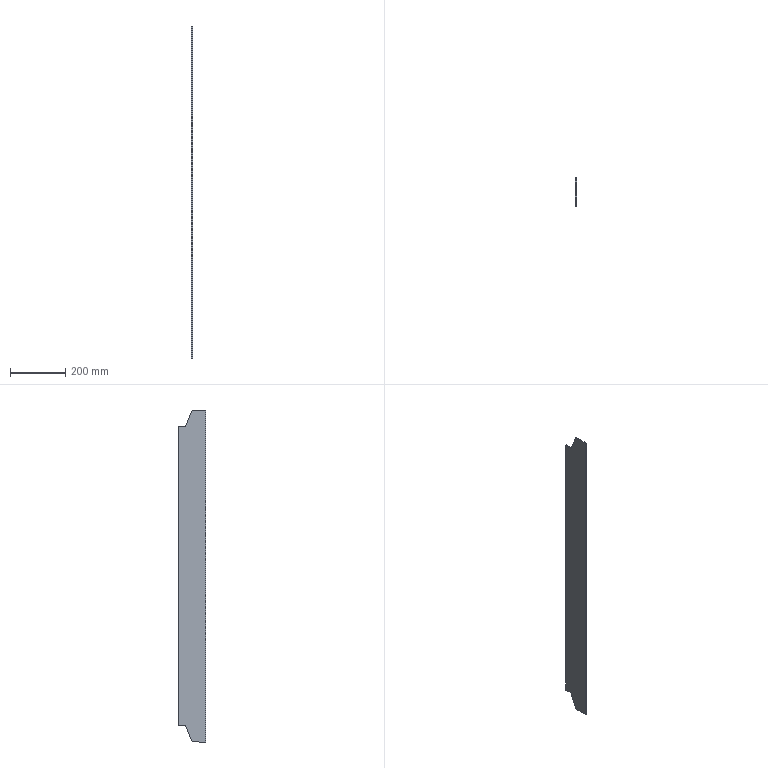Part | SolidWorks | features BaseBody 1 | 1 solid | 10 faces | box 3.795 x 101.02 x 1200 mm | volume 442400 mm3 | plane 9 | cylinder 1 | commonest cylinder face diameters 22.084 x1
STEP:
#1=CARTESIAN_POINT('',(-1.898,-111.897,-1200.));
#2=VERTEX_POINT('',#1);
#3=CARTESIAN_POINT('',(-1.898,-111.897,0.));
#4=VERTEX_POINT('',#3);
#5=CARTESIAN_POINT('',(-1.898,-111.897,0.));
#6=DIRECTION('',(0.,0.,1.));
#7=VECTOR('',#6,1000.);
#8=LINE('',#5,#7);
#9=EDGE_CURVE('',#2,#4,#8,.T.);
#10=ORIENTED_EDGE('',*,*,#9,.T.);
#11=CARTESIAN_POINT('',(-1.898,-61.387,0.));
#12=VERTEX_POINT('',#11);
#13=CARTESIAN_POINT('',(-1.898,-111.897,0.));
#14=DIRECTION('',(0.,1.,0.));
#15=VECTOR('',#14,1000.);
#16=LINE('',#13,#15);
#17=EDGE_CURVE('',#4,#12,#16,.T.);
#18=ORIENTED_EDGE('',*,*,#17,.T.);
#19=CARTESIAN_POINT('',(-1.898,-38.186,-58.335));
#20=VERTEX_POINT('',#19);
#21=CARTESIAN_POINT('',(-1.898,-61.387,0.));
#22=DIRECTION('',(0.,0.3696,-0.9292));
#23=VECTOR('',#22,1000.);
#24=LINE('',#21,#23);
#25=EDGE_CURVE('',#12,#20,#24,.T.);
#26=ORIENTED_EDGE('',*,*,#25,.T.);
#27=CARTESIAN_POINT('',(-1.898,-10.878,-58.335));
#28=VERTEX_POINT('',#27);
#29=CARTESIAN_POINT('',(-1.898,-111.897,-58.335));
#30=DIRECTION('',(0.,1.,0.));
#31=VECTOR('',#30,1000.);
#32=LINE('',#29,#31);
#33=EDGE_CURVE('',#20,#28,#32,.T.);
#34=ORIENTED_EDGE('',*,*,#33,.T.);
#35=CARTESIAN_POINT('',(-1.898,-10.878,-1141.665));
#36=VERTEX_POINT('',#35);
#37=CARTESIAN_POINT('',(-1.898,-10.878,0.));
#38=DIRECTION('',(0.,0.,-1.));
#39=VECTOR('',#38,1000.);
#40=LINE('',#37,#39);
#41=EDGE_CURVE('',#28,#36,#40,.T.);
#42=ORIENTED_EDGE('',*,*,#41,.T.);
#43=CARTESIAN_POINT('',(-1.898,-38.186,-1141.665));
#44=VERTEX_POINT('',#43);
#45=CARTESIAN_POINT('',(-1.898,-111.897,-1141.665));
#46=DIRECTION('',(0.,-1.,0.));
#47=VECTOR('',#46,1000.);
#48=LINE('',#45,#47);
#49=EDGE_CURVE('',#36,#44,#48,.T.);
#50=ORIENTED_EDGE('',*,*,#49,.T.);
#51=CARTESIAN_POINT('',(-1.898,-61.387,-1200.));
#52=VERTEX_POINT('',#51);
#53=CARTESIAN_POINT('',(-1.898,-38.186,-1141.665));
#54=DIRECTION('',(0.,-0.3696,-0.9292));
#55=VECTOR('',#54,1000.);
#56=LINE('',#53,#55);
#57=EDGE_CURVE('',#44,#52,#56,.T.);
#58=ORIENTED_EDGE('',*,*,#57,.T.);
#59=CARTESIAN_POINT('',(-1.898,-111.897,-1200.));
#60=DIRECTION('',(0.,-1.,0.));
#61=VECTOR('',#60,1000.);
#62=LINE('',#59,#61);
#63=EDGE_CURVE('',#52,#2,#62,.T.);
#64=ORIENTED_EDGE('',*,*,#63,.T.);
#65=EDGE_LOOP('',(#10,#18,#26,#34,#42,#50,#58,#64));
#66=FACE_OUTER_BOUND('',#65,.T.);
#67=CARTESIAN_POINT('',(-1.898,-111.897,0.));
#68=DIRECTION('',(-1.,0.,0.));
#69=DIRECTION('',(0.,-1.,0.));
#70=AXIS2_PLACEMENT_3D('',#67,#68,#69);
#71=PLANE('',#70);
#72=ADVANCED_FACE('',(#66),#71,.T.);
#73=CARTESIAN_POINT('',(1.898,-111.897,0.));
#74=VERTEX_POINT('',#73);
#75=CARTESIAN_POINT('',(0.,-111.897,0.));
#76=DIRECTION('',(1.,0.,0.));
#77=VECTOR('',#76,1000.);
#78=LINE('',#75,#77);
#79=EDGE_CURVE('',#4,#74,#78,.T.);
#80=ORIENTED_EDGE('',*,*,#79,.T.);
#81=CARTESIAN_POINT('',(1.898,-61.387,0.));
#82=VERTEX_POINT('',#81);
#83=CARTESIAN_POINT('',(1.898,-61.387,0.));
#84=DIRECTION('',(0.,1.,0.));
#85=VECTOR('',#84,1000.);
#86=LINE('',#83,#85);
#87=EDGE_CURVE('',#74,#82,#86,.T.);
#88=ORIENTED_EDGE('',*,*,#87,.T.);
#89=CARTESIAN_POINT('',(0.,-61.387,0.));
#90=DIRECTION('',(-1.,0.,0.));
#91=VECTOR('',#90,1000.);
#92=LINE('',#89,#91);
#93=EDGE_CURVE('',#82,#12,#92,.T.);
#94=ORIENTED_EDGE('',*,*,#93,.T.);
#95=ORIENTED_EDGE('',*,*,#17,.F.);
#96=EDGE_LOOP('',(#80,#88,#94,#95));
#97=FACE_OUTER_BOUND('',#96,.T.);
#98=CARTESIAN_POINT('',(0.,-61.387,0.));
#99=DIRECTION('',(0.,0.,1.));
#100=DIRECTION('',(1.,0.,0.));
#101=AXIS2_PLACEMENT_3D('',#98,#99,#100);
#102=PLANE('',#101);
#103=ADVANCED_FACE('',(#97),#102,.T.);
#104=CARTESIAN_POINT('',(1.898,-111.897,-1200.));
#105=VERTEX_POINT('',#104);
#106=CARTESIAN_POINT('',(1.898,-111.897,-1200.));
#107=DIRECTION('',(1.,0.,0.));
#108=VECTOR('',#107,1000.);
#109=LINE('',#106,#108);
#110=EDGE_CURVE('',#2,#105,#109,.T.);
#111=ORIENTED_EDGE('',*,*,#110,.T.);
#112=CARTESIAN_POINT('',(1.898,-111.897,0.));
#113=DIRECTION('',(0.,0.,1.));
#114=VECTOR('',#113,1000.);
#115=LINE('',#112,#114);
#116=EDGE_CURVE('',#105,#74,#115,.T.);
#117=ORIENTED_EDGE('',*,*,#116,.T.);
#118=ORIENTED_EDGE('',*,*,#79,.F.);
#119=ORIENTED_EDGE('',*,*,#9,.F.);
#120=EDGE_LOOP('',(#111,#117,#118,#119));
#121=FACE_OUTER_BOUND('',#120,.T.);
#122=CARTESIAN_POINT('',(1.898,-111.897,0.));
#123=DIRECTION('',(0.,-1.,0.));
#124=DIRECTION('',(0.,0.,-1.));
#125=AXIS2_PLACEMENT_3D('',#122,#123,#124);
#126=PLANE('',#125);
#127=ADVANCED_FACE('',(#121),#126,.T.);
#128=CARTESIAN_POINT('',(1.898,-61.387,-1200.));
#129=VERTEX_POINT('',#128);
#130=CARTESIAN_POINT('',(1.898,-61.387,-1200.));
#131=DIRECTION('',(0.,1.,0.));
#132=VECTOR('',#131,1000.);
#133=LINE('',#130,#132);
#134=EDGE_CURVE('',#105,#129,#133,.T.);
#135=ORIENTED_EDGE('',*,*,#134,.F.);
#136=ORIENTED_EDGE('',*,*,#110,.F.);
#137=ORIENTED_EDGE('',*,*,#63,.F.);
#138=CARTESIAN_POINT('',(0.,-61.387,-1200.));
#139=DIRECTION('',(-1.,0.,0.));
#140=VECTOR('',#139,1000.);
#141=LINE('',#138,#140);
#142=EDGE_CURVE('',#129,#52,#141,.T.);
#143=ORIENTED_EDGE('',*,*,#142,.F.);
#144=EDGE_LOOP('',(#135,#136,#137,#143));
#145=FACE_OUTER_BOUND('',#144,.T.);
#146=CARTESIAN_POINT('',(0.,-61.387,-1200.));
#147=DIRECTION('',(0.,0.,1.));
#148=DIRECTION('',(1.,0.,0.));
#149=AXIS2_PLACEMENT_3D('',#146,#147,#148);
#150=PLANE('',#149);
#151=ADVANCED_FACE('',(#145),#150,.F.);
#152=ORIENTED_EDGE('',*,*,#142,.T.);
#153=ORIENTED_EDGE('',*,*,#57,.F.);
#154=CARTESIAN_POINT('',(1.898,-38.186,-1141.665));
#155=VERTEX_POINT('',#154);
#156=CARTESIAN_POINT('',(-1.898,-38.186,-1141.665));
#157=DIRECTION('',(-1.,0.,0.));
#158=VECTOR('',#157,1000.);
#159=LINE('',#156,#158);
#160=EDGE_CURVE('',#155,#44,#159,.T.);
#161=ORIENTED_EDGE('',*,*,#160,.F.);
#162=CARTESIAN_POINT('',(1.898,-38.186,-1141.665));
#163=DIRECTION('',(0.,0.3696,0.9292));
#164=VECTOR('',#163,1000.);
#165=LINE('',#162,#164);
#166=EDGE_CURVE('',#129,#155,#165,.T.);
#167=ORIENTED_EDGE('',*,*,#166,.F.);
#168=EDGE_LOOP('',(#152,#153,#161,#167));
#169=FACE_OUTER_BOUND('',#168,.T.);
#170=CARTESIAN_POINT('',(-1.898,-38.186,-1141.665));
#171=DIRECTION('',(0.,-0.9292,0.3696));
#172=DIRECTION('',(0.,-0.3696,-0.9292));
#173=AXIS2_PLACEMENT_3D('',#170,#171,#172);
#174=PLANE('',#173);
#175=ADVANCED_FACE('',(#169),#174,.F.);
#176=ORIENTED_EDGE('',*,*,#160,.T.);
#177=ORIENTED_EDGE('',*,*,#49,.F.);
#178=CARTESIAN_POINT('',(1.898,-10.878,-1141.665));
#179=VERTEX_POINT('',#178);
#180=CARTESIAN_POINT('',(0.,0.,-1141.665));
#181=DIRECTION('',(0.,0.,-1.));
#182=DIRECTION('',(-1.,0.,0.));
#183=AXIS2_PLACEMENT_3D('',#180,#181,#182);
#184=CIRCLE('',#183,11.042);
#185=EDGE_CURVE('',#179,#36,#184,.T.);
#186=ORIENTED_EDGE('',*,*,#185,.F.);
#187=CARTESIAN_POINT('',(1.898,-10.878,-1141.665));
#188=DIRECTION('',(0.,1.,0.));
#189=VECTOR('',#188,1000.);
#190=LINE('',#187,#189);
#191=EDGE_CURVE('',#155,#179,#190,.T.);
#192=ORIENTED_EDGE('',*,*,#191,.F.);
#193=EDGE_LOOP('',(#176,#177,#186,#192));
#194=FACE_OUTER_BOUND('',#193,.T.);
#195=CARTESIAN_POINT('',(-1.898,-10.878,-1141.665));
#196=DIRECTION('',(0.,0.,1.));
#197=DIRECTION('',(1.,0.,0.));
#198=AXIS2_PLACEMENT_3D('',#195,#196,#197);
#199=PLANE('',#198);
#200=ADVANCED_FACE('',(#194),#199,.F.);
#201=CARTESIAN_POINT('',(1.898,-10.878,-58.335));
#202=VERTEX_POINT('',#201);
#203=CARTESIAN_POINT('',(1.898,-10.878,0.));
#204=DIRECTION('',(0.,0.,1.));
#205=VECTOR('',#204,1000.);
#206=LINE('',#203,#205);
#207=EDGE_CURVE('',#179,#202,#206,.T.);
#208=ORIENTED_EDGE('',*,*,#207,.F.);
#209=ORIENTED_EDGE('',*,*,#185,.T.);
#210=ORIENTED_EDGE('',*,*,#41,.F.);
#211=CARTESIAN_POINT('',(0.,0.,-58.335));
#212=DIRECTION('',(0.,0.,-1.));
#213=DIRECTION('',(-1.,0.,0.));
#214=AXIS2_PLACEMENT_3D('',#211,#212,#213);
#215=CIRCLE('',#214,11.042);
#216=EDGE_CURVE('',#202,#28,#215,.T.);
#217=ORIENTED_EDGE('',*,*,#216,.F.);
#218=EDGE_LOOP('',(#208,#209,#210,#217));
#219=FACE_OUTER_BOUND('',#218,.T.);
#220=CARTESIAN_POINT('',(0.,0.,0.));
#221=DIRECTION('',(0.,0.,-1.));
#222=DIRECTION('',(-1.,0.,0.));
#223=AXIS2_PLACEMENT_3D('',#220,#221,#222);
#224=CYLINDRICAL_SURFACE('',#223,11.042);
#225=ADVANCED_FACE('',(#219),#224,.F.);
#226=ORIENTED_EDGE('',*,*,#216,.T.);
#227=ORIENTED_EDGE('',*,*,#33,.F.);
#228=CARTESIAN_POINT('',(1.898,-38.186,-58.335));
#229=VERTEX_POINT('',#228);
#230=CARTESIAN_POINT('',(-1.898,-38.186,-58.335));
#231=DIRECTION('',(-1.,0.,0.));
#232=VECTOR('',#231,1000.);
#233=LINE('',#230,#232);
#234=EDGE_CURVE('',#229,#20,#233,.T.);
#235=ORIENTED_EDGE('',*,*,#234,.F.);
#236=CARTESIAN_POINT('',(1.898,-38.186,-58.335));
#237=DIRECTION('',(0.,-1.,0.));
#238=VECTOR('',#237,1000.);
#239=LINE('',#236,#238);
#240=EDGE_CURVE('',#202,#229,#239,.T.);
#241=ORIENTED_EDGE('',*,*,#240,.F.);
#242=EDGE_LOOP('',(#226,#227,#235,#241));
#243=FACE_OUTER_BOUND('',#242,.T.);
#244=CARTESIAN_POINT('',(-1.898,-38.186,-58.335));
#245=DIRECTION('',(0.,0.,-1.));
#246=DIRECTION('',(-1.,0.,0.));
#247=AXIS2_PLACEMENT_3D('',#244,#245,#246);
#248=PLANE('',#247);
#249=ADVANCED_FACE('',(#243),#248,.F.);
#250=ORIENTED_EDGE('',*,*,#234,.T.);
#251=ORIENTED_EDGE('',*,*,#25,.F.);
#252=ORIENTED_EDGE('',*,*,#93,.F.);
#253=CARTESIAN_POINT('',(1.898,-61.387,0.));
#254=DIRECTION('',(0.,-0.3696,0.9292));
#255=VECTOR('',#254,1000.);
#256=LINE('',#253,#255);
#257=EDGE_CURVE('',#229,#82,#256,.T.);
#258=ORIENTED_EDGE('',*,*,#257,.F.);
#259=EDGE_LOOP('',(#250,#251,#252,#258));
#260=FACE_OUTER_BOUND('',#259,.T.);
#261=CARTESIAN_POINT('',(-1.898,-61.387,0.));
#262=DIRECTION('',(0.,-0.9292,-0.3696));
#263=DIRECTION('',(0.,0.3696,-0.9292));
#264=AXIS2_PLACEMENT_3D('',#261,#262,#263);
#265=PLANE('',#264);
#266=ADVANCED_FACE('',(#260),#265,.F.);
#267=ORIENTED_EDGE('',*,*,#191,.T.);
#268=ORIENTED_EDGE('',*,*,#207,.T.);
#269=ORIENTED_EDGE('',*,*,#240,.T.);
#270=ORIENTED_EDGE('',*,*,#257,.T.);
#271=ORIENTED_EDGE('',*,*,#87,.F.);
#272=ORIENTED_EDGE('',*,*,#116,.F.);
#273=ORIENTED_EDGE('',*,*,#134,.T.);
#274=ORIENTED_EDGE('',*,*,#166,.T.);
#275=EDGE_LOOP('',(#267,#268,#269,#270,#271,#272,#273,#274));
#276=FACE_OUTER_BOUND('',#275,.T.);
#277=CARTESIAN_POINT('',(1.898,-10.878,0.));
#278=DIRECTION('',(1.,0.,0.));
#279=DIRECTION('',(0.,1.,0.));
#280=AXIS2_PLACEMENT_3D('',#277,#278,#279);
#281=PLANE('',#280);
#282=ADVANCED_FACE('',(#276),#281,.T.);
#283=CLOSED_SHELL('',(#72,#103,#127,#151,#175,#200,#225,#249,#266,#282));
#284=MANIFOLD_SOLID_BREP('',#283);
#285=CARTESIAN_POINT('',(0.,0.,0.));
#286=DIRECTION('',(0.,0.,1.));
#287=DIRECTION('',(1.,0.,0.));
#288=AXIS2_PLACEMENT_3D('',#285,#286,#287);
#289=(LENGTH_UNIT()NAMED_UNIT(*)SI_UNIT(.MILLI.,.METRE.));
#290=UNCERTAINTY_MEASURE_WITH_UNIT(LENGTH_MEASURE(0.00001),#289,'','');
#291=(NAMED_UNIT(*)PLANE_ANGLE_UNIT()SI_UNIT($,.RADIAN.));
#292=(NAMED_UNIT(*)SI_UNIT($,.STERADIAN.)SOLID_ANGLE_UNIT());
#293=(GEOMETRIC_REPRESENTATION_CONTEXT(3)GLOBAL_UNCERTAINTY_ASSIGNED_CONTEXT((#290))GLOBAL_UNIT_ASSIGNED_CONTEXT((#289,#291,#292))REPRESENTATION_CONTEXT('',''));
#294=ADVANCED_BREP_SHAPE_REPRESENTATION('',(#284,#288),#293);